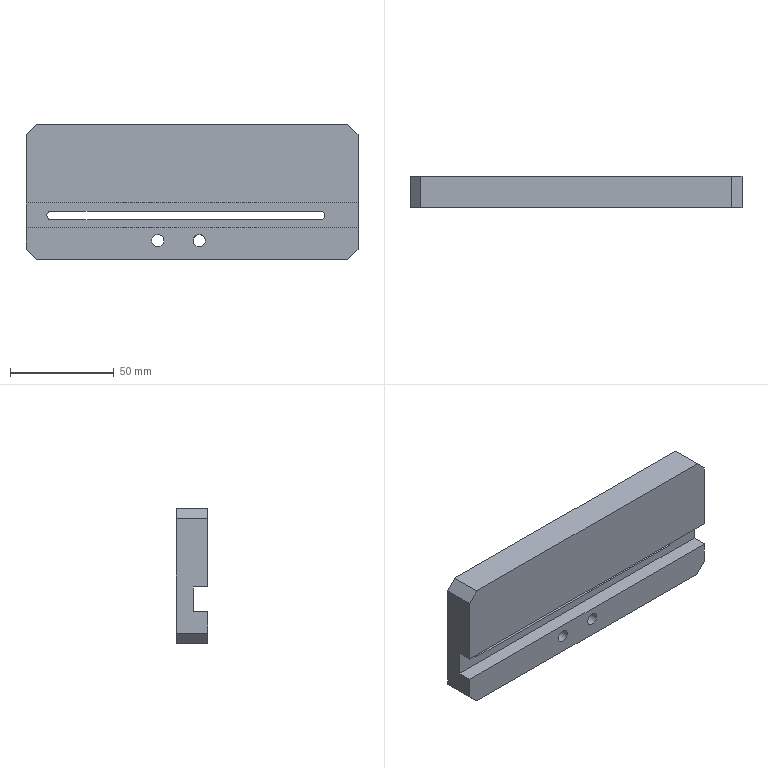Part | STEP file | solid 48 | 1 solid | 24 faces | box 160 x 15 x 65 mm | volume 135897 mm3 | plane 18 | cylinder 6 | commonest cylinder face diameters 4 x2 6 x2 10 x2